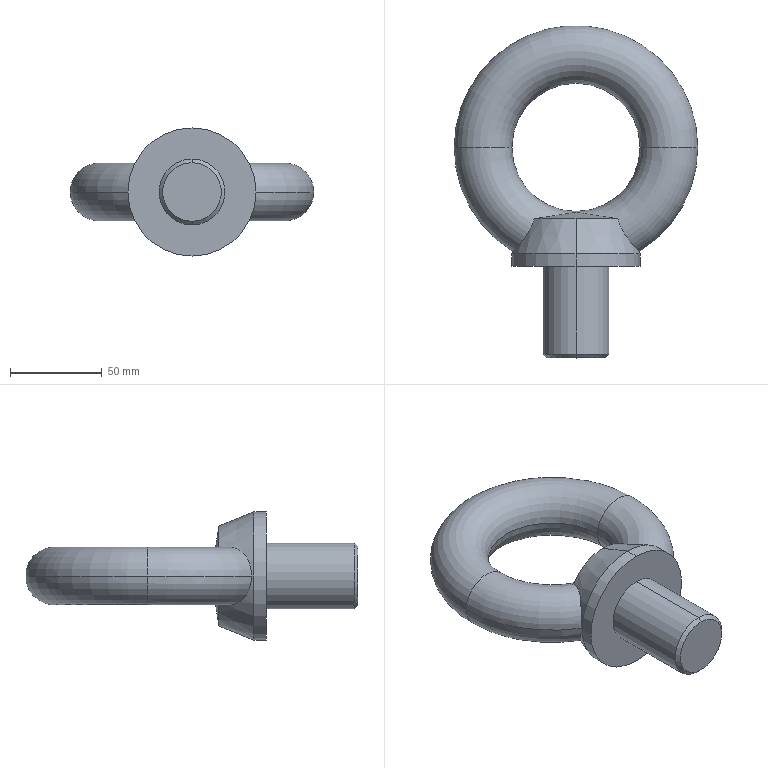Part | Creo | 1 solid | 16 faces | box 133 x 181.5 x 70 mm | volume 345866 mm3 | cone 6 | torus 4 | cylinder 4 | plane 2 | commonest cylinder face diameters 36 x2 70 x2
STEP:
#1=CARTESIAN_POINT('',(-22.859,376.,-80.242));
#2=VERTEX_POINT('',#1);
#3=CARTESIAN_POINT('',(0.,379.333,-70.034));
#4=VERTEX_POINT('',#3);
#5=CARTESIAN_POINT('',(-22.859,376.,-80.242));
#6=CARTESIAN_POINT('',(-21.93,376.132,-80.022));
#7=CARTESIAN_POINT('',(-20.175,376.386,-79.542));
#8=CARTESIAN_POINT('',(-17.843,376.731,-78.764));
#9=CARTESIAN_POINT('',(-15.766,377.045,-77.963));
#10=CARTESIAN_POINT('',(-13.906,377.331,-77.165));
#11=CARTESIAN_POINT('',(-12.241,377.591,-76.387));
#12=CARTESIAN_POINT('',(-10.742,377.828,-75.639));
#13=CARTESIAN_POINT('',(-9.385,378.044,-74.925));
#14=CARTESIAN_POINT('',(-8.149,378.242,-74.246));
#15=CARTESIAN_POINT('',(-7.011,378.425,-73.6));
#16=CARTESIAN_POINT('',(-5.956,378.594,-72.984));
#17=CARTESIAN_POINT('',(-4.977,378.75,-72.398));
#18=CARTESIAN_POINT('',(-4.073,378.891,-71.851));
#19=CARTESIAN_POINT('',(-3.245,379.016,-71.359));
#20=CARTESIAN_POINT('',(-2.502,379.122,-70.928));
#21=CARTESIAN_POINT('',(-1.815,379.213,-70.544));
#22=CARTESIAN_POINT('',(-1.153,379.284,-70.244));
#23=CARTESIAN_POINT('',(-0.5447,379.325,-70.071));
#24=CARTESIAN_POINT('',(-0.1835,379.333,-70.034));
#25=B_SPLINE_CURVE_WITH_KNOTS('',3,(#5,#6,#7,#8,#9,#10,#11,#12,#13,#14,#15,#16,#17,#18,#19,#20,#21,#22,#23,#24,#3),.UNSPECIFIED.,.F.,.F.,(4,1,1,1,1,1,1,1,1,1,1,1,1,1,1,1,1,1,4),(0.,0.05556,0.1111,0.1667,0.2222,0.2778,0.3333,0.3889,0.4444,0.5,0.5556,0.6111,0.6667,0.7222,0.7778,0.8333,0.8889,0.9444,1.),.UNSPECIFIED.);
#26=EDGE_CURVE('',#2,#4,#25,.T.);
#27=ORIENTED_EDGE('',*,*,#26,.F.);
#28=CARTESIAN_POINT('',(0.,376.,-92.7));
#29=VERTEX_POINT('',#28);
#30=CARTESIAN_POINT('',(0.,376.,-65.5));
#31=DIRECTION('',(0.,-1.,0.));
#32=DIRECTION('',(-0.8404,0.,-0.542));
#33=AXIS2_PLACEMENT_3D('',#30,#31,#32);
#34=CIRCLE('',#33,27.2);
#35=EDGE_CURVE('',#2,#29,#34,.T.);
#36=ORIENTED_EDGE('',*,*,#35,.T.);
#37=CARTESIAN_POINT('',(22.859,376.,-80.242));
#38=VERTEX_POINT('',#37);
#39=CARTESIAN_POINT('',(0.,376.,-65.5));
#40=DIRECTION('',(0.,-1.,0.));
#41=DIRECTION('',(0.,0.,-1.));
#42=AXIS2_PLACEMENT_3D('',#39,#40,#41);
#43=CIRCLE('',#42,27.2);
#44=EDGE_CURVE('',#29,#38,#43,.T.);
#45=ORIENTED_EDGE('',*,*,#44,.T.);
#46=CARTESIAN_POINT('',(0.,379.333,-70.034));
#47=CARTESIAN_POINT('',(0.1802,379.333,-70.034));
#48=CARTESIAN_POINT('',(0.5342,379.325,-70.071));
#49=CARTESIAN_POINT('',(1.137,379.283,-70.25));
#50=CARTESIAN_POINT('',(1.772,379.216,-70.538));
#51=CARTESIAN_POINT('',(2.453,379.129,-70.899));
#52=CARTESIAN_POINT('',(3.203,379.022,-71.335));
#53=CARTESIAN_POINT('',(4.029,378.898,-71.826));
#54=CARTESIAN_POINT('',(4.932,378.757,-72.37));
#55=CARTESIAN_POINT('',(5.909,378.601,-72.956));
#56=CARTESIAN_POINT('',(6.96,378.433,-73.571));
#57=CARTESIAN_POINT('',(8.095,378.251,-74.217));
#58=CARTESIAN_POINT('',(9.329,378.053,-74.896));
#59=CARTESIAN_POINT('',(10.686,377.837,-75.611));
#60=CARTESIAN_POINT('',(12.188,377.6,-76.362));
#61=CARTESIAN_POINT('',(13.857,377.339,-77.144));
#62=CARTESIAN_POINT('',(15.725,377.051,-77.948));
#63=CARTESIAN_POINT('',(17.811,376.736,-78.754));
#64=CARTESIAN_POINT('',(20.155,376.389,-79.537));
#65=CARTESIAN_POINT('',(21.923,376.133,-80.021));
#66=CARTESIAN_POINT('',(22.859,376.,-80.242));
#67=B_SPLINE_CURVE_WITH_KNOTS('',3,(#46,#47,#48,#49,#50,#51,#52,#53,#54,#55,#56,#57,#58,#59,#60,#61,#62,#63,#64,#65,#66),.UNSPECIFIED.,.F.,.F.,(4,1,1,1,1,1,1,1,1,1,1,1,1,1,1,1,1,1,4),(0.,0.05556,0.1111,0.1667,0.2222,0.2778,0.3333,0.3889,0.4444,0.5,0.5556,0.6111,0.6667,0.7222,0.7778,0.8333,0.8889,0.9444,1.),.UNSPECIFIED.);
#68=EDGE_CURVE('',#4,#38,#67,.T.);
#69=ORIENTED_EDGE('',*,*,#68,.F.);
#70=EDGE_LOOP('',(#27,#36,#45,#69));
#71=FACE_OUTER_BOUND('',#70,.F.);
#72=CARTESIAN_POINT('',(0.,377.667,-65.5));
#73=DIRECTION('',(0.,-1.,0.));
#74=DIRECTION('',(0.,0.,-1.));
#75=AXIS2_PLACEMENT_3D('',#72,#73,#74);
#76=CONICAL_SURFACE('',#75,15.867,81.634);
#77=ADVANCED_FACE('',(#71),#76,.T.);
#78=CARTESIAN_POINT('',(34.464,358.128,-65.5));
#79=VERTEX_POINT('',#78);
#80=CARTESIAN_POINT('',(22.859,376.,-80.242));
#81=CARTESIAN_POINT('',(23.041,375.255,-80.518));
#82=CARTESIAN_POINT('',(23.475,373.76,-80.963));
#83=CARTESIAN_POINT('',(24.371,371.476,-81.291));
#84=CARTESIAN_POINT('',(25.482,369.249,-81.233));
#85=CARTESIAN_POINT('',(26.763,367.124,-80.777));
#86=CARTESIAN_POINT('',(28.132,365.163,-79.93));
#87=CARTESIAN_POINT('',(29.531,363.381,-78.699));
#88=CARTESIAN_POINT('',(30.873,361.82,-77.114));
#89=CARTESIAN_POINT('',(32.081,360.511,-75.22));
#90=CARTESIAN_POINT('',(33.099,359.464,-73.055));
#91=CARTESIAN_POINT('',(33.871,358.7,-70.672));
#92=CARTESIAN_POINT('',(34.354,358.233,-68.128));
#93=CARTESIAN_POINT('',(34.464,358.128,-66.381));
#94=CARTESIAN_POINT('',(34.464,358.128,-65.5));
#95=B_SPLINE_CURVE_WITH_KNOTS('',3,(#80,#81,#82,#83,#84,#85,#86,#87,#88,#89,#90,#91,#92,#93,#94),.UNSPECIFIED.,.F.,.F.,(4,1,1,1,1,1,1,1,1,1,1,1,4),(0.,0.08333,0.1667,0.25,0.3333,0.4167,0.5,0.5833,0.6667,0.75,0.8333,0.9167,1.),.UNSPECIFIED.);
#96=EDGE_CURVE('',#38,#79,#95,.T.);
#97=ORIENTED_EDGE('',*,*,#96,.T.);
#98=CARTESIAN_POINT('',(66.5,415.,-65.5));
#99=VERTEX_POINT('',#98);
#100=CARTESIAN_POINT('',(0.,415.,-65.5));
#101=DIRECTION('',(0.,0.,1.));
#102=DIRECTION('',(0.5183,-0.8552,0.));
#103=AXIS2_PLACEMENT_3D('',#100,#101,#102);
#104=CIRCLE('',#103,66.5);
#105=EDGE_CURVE('',#79,#99,#104,.T.);
#106=ORIENTED_EDGE('',*,*,#105,.T.);
#107=CARTESIAN_POINT('',(35.,415.,-65.5));
#108=VERTEX_POINT('',#107);
#109=CARTESIAN_POINT('',(50.75,415.,-65.5));
#110=DIRECTION('',(0.,-1.,0.));
#111=DIRECTION('',(-1.,0.,0.));
#112=AXIS2_PLACEMENT_3D('',#109,#110,#111);
#113=CIRCLE('',#112,15.75);
#114=EDGE_CURVE('',#108,#99,#113,.T.);
#115=ORIENTED_EDGE('',*,*,#114,.F.);
#116=CARTESIAN_POINT('',(-35.,415.,-65.5));
#117=VERTEX_POINT('',#116);
#118=CARTESIAN_POINT('',(0.,415.,-65.5));
#119=DIRECTION('',(0.,0.,1.));
#120=DIRECTION('',(-1.,0.,0.));
#121=AXIS2_PLACEMENT_3D('',#118,#119,#120);
#122=CIRCLE('',#121,35.);
#123=EDGE_CURVE('',#117,#108,#122,.T.);
#124=ORIENTED_EDGE('',*,*,#123,.F.);
#125=CARTESIAN_POINT('',(-66.5,415.,-65.5));
#126=VERTEX_POINT('',#125);
#127=CARTESIAN_POINT('',(-50.75,415.,-65.5));
#128=DIRECTION('',(0.,1.,0.));
#129=DIRECTION('',(1.,0.,0.));
#130=AXIS2_PLACEMENT_3D('',#127,#128,#129);
#131=CIRCLE('',#130,15.75);
#132=EDGE_CURVE('',#117,#126,#131,.T.);
#133=ORIENTED_EDGE('',*,*,#132,.T.);
#134=CARTESIAN_POINT('',(-34.464,358.128,-65.5));
#135=VERTEX_POINT('',#134);
#136=CARTESIAN_POINT('',(0.,415.,-65.5));
#137=DIRECTION('',(0.,0.,1.));
#138=DIRECTION('',(-1.,0.,0.));
#139=AXIS2_PLACEMENT_3D('',#136,#137,#138);
#140=CIRCLE('',#139,66.5);
#141=EDGE_CURVE('',#126,#135,#140,.T.);
#142=ORIENTED_EDGE('',*,*,#141,.T.);
#143=CARTESIAN_POINT('',(-34.464,358.128,-65.5));
#144=CARTESIAN_POINT('',(-34.464,358.128,-66.375));
#145=CARTESIAN_POINT('',(-34.356,358.232,-68.112));
#146=CARTESIAN_POINT('',(-33.877,358.694,-70.647));
#147=CARTESIAN_POINT('',(-33.11,359.453,-73.027));
#148=CARTESIAN_POINT('',(-32.096,360.495,-75.192));
#149=CARTESIAN_POINT('',(-30.893,361.798,-77.086));
#150=CARTESIAN_POINT('',(-29.558,363.349,-78.672));
#151=CARTESIAN_POINT('',(-28.158,365.129,-79.912));
#152=CARTESIAN_POINT('',(-26.777,367.1,-80.771));
#153=CARTESIAN_POINT('',(-25.488,369.238,-81.232));
#154=CARTESIAN_POINT('',(-24.374,371.47,-81.291));
#155=CARTESIAN_POINT('',(-23.476,373.757,-80.964));
#156=CARTESIAN_POINT('',(-23.041,375.253,-80.519));
#157=CARTESIAN_POINT('',(-22.859,376.,-80.242));
#158=B_SPLINE_CURVE_WITH_KNOTS('',3,(#143,#144,#145,#146,#147,#148,#149,#150,#151,#152,#153,#154,#155,#156,#157),.UNSPECIFIED.,.F.,.F.,(4,1,1,1,1,1,1,1,1,1,1,1,4),(0.,0.08333,0.1667,0.25,0.3333,0.4167,0.5,0.5833,0.6667,0.75,0.8333,0.9167,1.),.UNSPECIFIED.);
#159=EDGE_CURVE('',#135,#2,#158,.T.);
#160=ORIENTED_EDGE('',*,*,#159,.T.);
#161=ORIENTED_EDGE('',*,*,#26,.T.);
#162=ORIENTED_EDGE('',*,*,#68,.T.);
#163=EDGE_LOOP('',(#97,#106,#115,#124,#133,#142,#160,#161,#162));
#164=FACE_OUTER_BOUND('',#163,.F.);
#165=CARTESIAN_POINT('',(0.,415.,-65.5));
#166=DIRECTION('',(0.,0.,1.));
#167=DIRECTION('',(1.,0.,0.));
#168=AXIS2_PLACEMENT_3D('',#165,#166,#167);
#169=TOROIDAL_SURFACE('',#168,50.75,15.75);
#170=ADVANCED_FACE('',(#164),#169,.T.);
#171=ORIENTED_EDGE('',*,*,#96,.F.);
#172=ORIENTED_EDGE('',*,*,#44,.F.);
#173=CARTESIAN_POINT('',(0.,356.81,-100.5));
#174=VERTEX_POINT('',#173);
#175=CARTESIAN_POINT('',(0.,376.,-92.7));
#176=DIRECTION('',(0.,-0.9264,-0.3765));
#177=VECTOR('',#176,20.715);
#178=LINE('',#175,#177);
#179=EDGE_CURVE('',#29,#174,#178,.T.);
#180=ORIENTED_EDGE('',*,*,#179,.T.);
#181=CARTESIAN_POINT('',(0.,356.81,-30.5));
#182=VERTEX_POINT('',#181);
#183=CARTESIAN_POINT('',(0.,356.81,-65.5));
#184=DIRECTION('',(0.,1.,0.));
#185=DIRECTION('',(0.,0.,1.));
#186=AXIS2_PLACEMENT_3D('',#183,#184,#185);
#187=CIRCLE('',#186,35.);
#188=EDGE_CURVE('',#182,#174,#187,.T.);
#189=ORIENTED_EDGE('',*,*,#188,.F.);
#190=CARTESIAN_POINT('',(0.,376.,-38.3));
#191=VERTEX_POINT('',#190);
#192=CARTESIAN_POINT('',(0.,376.,-38.3));
#193=DIRECTION('',(0.,-0.9264,0.3765));
#194=VECTOR('',#193,20.715);
#195=LINE('',#192,#194);
#196=EDGE_CURVE('',#191,#182,#195,.T.);
#197=ORIENTED_EDGE('',*,*,#196,.F.);
#198=CARTESIAN_POINT('',(22.859,376.,-50.758));
#199=VERTEX_POINT('',#198);
#200=CARTESIAN_POINT('',(0.,376.,-65.5));
#201=DIRECTION('',(0.,-1.,0.));
#202=DIRECTION('',(0.8404,0.,0.542));
#203=AXIS2_PLACEMENT_3D('',#200,#201,#202);
#204=CIRCLE('',#203,27.2);
#205=EDGE_CURVE('',#199,#191,#204,.T.);
#206=ORIENTED_EDGE('',*,*,#205,.F.);
#207=CARTESIAN_POINT('',(34.464,358.128,-65.5));
#208=CARTESIAN_POINT('',(34.464,358.128,-64.625));
#209=CARTESIAN_POINT('',(34.356,358.232,-62.888));
#210=CARTESIAN_POINT('',(33.877,358.694,-60.353));
#211=CARTESIAN_POINT('',(33.11,359.453,-57.973));
#212=CARTESIAN_POINT('',(32.096,360.495,-55.808));
#213=CARTESIAN_POINT('',(30.893,361.798,-53.914));
#214=CARTESIAN_POINT('',(29.558,363.349,-52.328));
#215=CARTESIAN_POINT('',(28.158,365.129,-51.088));
#216=CARTESIAN_POINT('',(26.777,367.1,-50.229));
#217=CARTESIAN_POINT('',(25.488,369.238,-49.768));
#218=CARTESIAN_POINT('',(24.374,371.47,-49.709));
#219=CARTESIAN_POINT('',(23.476,373.757,-50.036));
#220=CARTESIAN_POINT('',(23.041,375.253,-50.481));
#221=CARTESIAN_POINT('',(22.859,376.,-50.758));
#222=B_SPLINE_CURVE_WITH_KNOTS('',3,(#207,#208,#209,#210,#211,#212,#213,#214,#215,#216,#217,#218,#219,#220,#221),.UNSPECIFIED.,.F.,.F.,(4,1,1,1,1,1,1,1,1,1,1,1,4),(0.,0.08333,0.1667,0.25,0.3333,0.4167,0.5,0.5833,0.6667,0.75,0.8333,0.9167,1.),.UNSPECIFIED.);
#223=EDGE_CURVE('',#79,#199,#222,.T.);
#224=ORIENTED_EDGE('',*,*,#223,.F.);
#225=EDGE_LOOP('',(#171,#172,#180,#189,#197,#206,#224));
#226=FACE_OUTER_BOUND('',#225,.F.);
#227=CARTESIAN_POINT('',(0.,366.405,-65.5));
#228=DIRECTION('',(0.,-1.,0.));
#229=DIRECTION('',(0.,0.,-1.));
#230=AXIS2_PLACEMENT_3D('',#227,#228,#229);
#231=CONICAL_SURFACE('',#230,31.1,22.12);
#232=ADVANCED_FACE('',(#226),#231,.T.);
#233=CARTESIAN_POINT('',(-22.859,376.,-50.758));
#234=VERTEX_POINT('',#233);
#235=CARTESIAN_POINT('',(0.,376.,-65.5));
#236=DIRECTION('',(0.,-1.,0.));
#237=DIRECTION('',(0.,0.,1.));
#238=AXIS2_PLACEMENT_3D('',#235,#236,#237);
#239=CIRCLE('',#238,27.2);
#240=EDGE_CURVE('',#191,#234,#239,.T.);
#241=ORIENTED_EDGE('',*,*,#240,.F.);
#242=ORIENTED_EDGE('',*,*,#196,.T.);
#243=CARTESIAN_POINT('',(0.,356.81,-65.5));
#244=DIRECTION('',(0.,1.,0.));
#245=DIRECTION('',(0.,0.,-1.));
#246=AXIS2_PLACEMENT_3D('',#243,#244,#245);
#247=CIRCLE('',#246,35.);
#248=EDGE_CURVE('',#174,#182,#247,.T.);
#249=ORIENTED_EDGE('',*,*,#248,.F.);
#250=ORIENTED_EDGE('',*,*,#179,.F.);
#251=ORIENTED_EDGE('',*,*,#35,.F.);
#252=ORIENTED_EDGE('',*,*,#159,.F.);
#253=CARTESIAN_POINT('',(-22.859,376.,-50.758));
#254=CARTESIAN_POINT('',(-23.041,375.255,-50.482));
#255=CARTESIAN_POINT('',(-23.475,373.76,-50.037));
#256=CARTESIAN_POINT('',(-24.371,371.476,-49.709));
#257=CARTESIAN_POINT('',(-25.482,369.249,-49.767));
#258=CARTESIAN_POINT('',(-26.763,367.124,-50.223));
#259=CARTESIAN_POINT('',(-28.132,365.163,-51.07));
#260=CARTESIAN_POINT('',(-29.531,363.381,-52.301));
#261=CARTESIAN_POINT('',(-30.873,361.82,-53.886));
#262=CARTESIAN_POINT('',(-32.081,360.511,-55.78));
#263=CARTESIAN_POINT('',(-33.099,359.464,-57.945));
#264=CARTESIAN_POINT('',(-33.871,358.7,-60.328));
#265=CARTESIAN_POINT('',(-34.354,358.233,-62.872));
#266=CARTESIAN_POINT('',(-34.464,358.128,-64.619));
#267=CARTESIAN_POINT('',(-34.464,358.128,-65.5));
#268=B_SPLINE_CURVE_WITH_KNOTS('',3,(#253,#254,#255,#256,#257,#258,#259,#260,#261,#262,#263,#264,#265,#266,#267),.UNSPECIFIED.,.F.,.F.,(4,1,1,1,1,1,1,1,1,1,1,1,4),(0.,0.08333,0.1667,0.25,0.3333,0.4167,0.5,0.5833,0.6667,0.75,0.8333,0.9167,1.),.UNSPECIFIED.);
#269=EDGE_CURVE('',#234,#135,#268,.T.);
#270=ORIENTED_EDGE('',*,*,#269,.F.);
#271=EDGE_LOOP('',(#241,#242,#249,#250,#251,#252,#270));
#272=FACE_OUTER_BOUND('',#271,.F.);
#273=CARTESIAN_POINT('',(0.,366.405,-65.5));
#274=DIRECTION('',(0.,-1.,0.));
#275=DIRECTION('',(0.,0.,-1.));
#276=AXIS2_PLACEMENT_3D('',#273,#274,#275);
#277=CONICAL_SURFACE('',#276,31.1,22.12);
#278=ADVANCED_FACE('',(#272),#277,.T.);
#279=CARTESIAN_POINT('',(0.,379.333,-60.966));
#280=VERTEX_POINT('',#279);
#281=CARTESIAN_POINT('',(22.859,376.,-50.758));
#282=CARTESIAN_POINT('',(21.93,376.132,-50.978));
#283=CARTESIAN_POINT('',(20.175,376.386,-51.458));
#284=CARTESIAN_POINT('',(17.843,376.731,-52.236));
#285=CARTESIAN_POINT('',(15.766,377.045,-53.037));
#286=CARTESIAN_POINT('',(13.906,377.331,-53.835));
#287=CARTESIAN_POINT('',(12.241,377.591,-54.613));
#288=CARTESIAN_POINT('',(10.742,377.828,-55.361));
#289=CARTESIAN_POINT('',(9.385,378.044,-56.075));
#290=CARTESIAN_POINT('',(8.149,378.242,-56.754));
#291=CARTESIAN_POINT('',(7.011,378.425,-57.4));
#292=CARTESIAN_POINT('',(5.956,378.594,-58.016));
#293=CARTESIAN_POINT('',(4.977,378.75,-58.602));
#294=CARTESIAN_POINT('',(4.073,378.891,-59.149));
#295=CARTESIAN_POINT('',(3.245,379.016,-59.641));
#296=CARTESIAN_POINT('',(2.502,379.122,-60.072));
#297=CARTESIAN_POINT('',(1.815,379.213,-60.456));
#298=CARTESIAN_POINT('',(1.153,379.284,-60.756));
#299=CARTESIAN_POINT('',(0.5447,379.325,-60.929));
#300=CARTESIAN_POINT('',(0.1835,379.333,-60.966));
#301=B_SPLINE_CURVE_WITH_KNOTS('',3,(#281,#282,#283,#284,#285,#286,#287,#288,#289,#290,#291,#292,#293,#294,#295,#296,#297,#298,#299,#300,#279),.UNSPECIFIED.,.F.,.F.,(4,1,1,1,1,1,1,1,1,1,1,1,1,1,1,1,1,1,4),(0.,0.05556,0.1111,0.1667,0.2222,0.2778,0.3333,0.3889,0.4444,0.5,0.5556,0.6111,0.6667,0.7222,0.7778,0.8333,0.8889,0.9444,1.),.UNSPECIFIED.);
#302=EDGE_CURVE('',#199,#280,#301,.T.);
#303=ORIENTED_EDGE('',*,*,#302,.F.);
#304=ORIENTED_EDGE('',*,*,#205,.T.);
#305=ORIENTED_EDGE('',*,*,#240,.T.);
#306=CARTESIAN_POINT('',(0.,379.333,-60.966));
#307=CARTESIAN_POINT('',(-0.1802,379.333,-60.966));
#308=CARTESIAN_POINT('',(-0.5342,379.325,-60.929));
#309=CARTESIAN_POINT('',(-1.137,379.283,-60.75));
#310=CARTESIAN_POINT('',(-1.772,379.216,-60.462));
#311=CARTESIAN_POINT('',(-2.453,379.129,-60.101));
#312=CARTESIAN_POINT('',(-3.203,379.022,-59.665));
#313=CARTESIAN_POINT('',(-4.029,378.898,-59.174));
#314=CARTESIAN_POINT('',(-4.932,378.757,-58.63));
#315=CARTESIAN_POINT('',(-5.909,378.601,-58.044));
#316=CARTESIAN_POINT('',(-6.96,378.433,-57.429));
#317=CARTESIAN_POINT('',(-8.095,378.251,-56.783));
#318=CARTESIAN_POINT('',(-9.329,378.053,-56.104));
#319=CARTESIAN_POINT('',(-10.686,377.837,-55.389));
#320=CARTESIAN_POINT('',(-12.188,377.6,-54.638));
#321=CARTESIAN_POINT('',(-13.857,377.339,-53.856));
#322=CARTESIAN_POINT('',(-15.725,377.051,-53.052));
#323=CARTESIAN_POINT('',(-17.811,376.736,-52.246));
#324=CARTESIAN_POINT('',(-20.155,376.389,-51.463));
#325=CARTESIAN_POINT('',(-21.923,376.133,-50.979));
#326=CARTESIAN_POINT('',(-22.859,376.,-50.758));
#327=B_SPLINE_CURVE_WITH_KNOTS('',3,(#306,#307,#308,#309,#310,#311,#312,#313,#314,#315,#316,#317,#318,#319,#320,#321,#322,#323,#324,#325,#326),.UNSPECIFIED.,.F.,.F.,(4,1,1,1,1,1,1,1,1,1,1,1,1,1,1,1,1,1,4),(0.,0.05556,0.1111,0.1667,0.2222,0.2778,0.3333,0.3889,0.4444,0.5,0.5556,0.6111,0.6667,0.7222,0.7778,0.8333,0.8889,0.9444,1.),.UNSPECIFIED.);
#328=EDGE_CURVE('',#280,#234,#327,.T.);
#329=ORIENTED_EDGE('',*,*,#328,.F.);
#330=EDGE_LOOP('',(#303,#304,#305,#329));
#331=FACE_OUTER_BOUND('',#330,.F.);
#332=CARTESIAN_POINT('',(0.,377.667,-65.5));
#333=DIRECTION('',(0.,-1.,0.));
#334=DIRECTION('',(0.,0.,-1.));
#335=AXIS2_PLACEMENT_3D('',#332,#333,#334);
#336=CONICAL_SURFACE('',#335,15.867,81.634);
#337=ADVANCED_FACE('',(#331),#336,.T.);
#338=ORIENTED_EDGE('',*,*,#223,.T.);
#339=ORIENTED_EDGE('',*,*,#302,.T.);
#340=ORIENTED_EDGE('',*,*,#328,.T.);
#341=ORIENTED_EDGE('',*,*,#269,.T.);
#342=ORIENTED_EDGE('',*,*,#141,.F.);
#343=CARTESIAN_POINT('',(-50.75,415.,-65.5));
#344=DIRECTION('',(0.,1.,0.));
#345=DIRECTION('',(-1.,0.,0.));
#346=AXIS2_PLACEMENT_3D('',#343,#344,#345);
#347=CIRCLE('',#346,15.75);
#348=EDGE_CURVE('',#126,#117,#347,.T.);
#349=ORIENTED_EDGE('',*,*,#348,.T.);
#350=ORIENTED_EDGE('',*,*,#123,.T.);
#351=CARTESIAN_POINT('',(50.75,415.,-65.5));
#352=DIRECTION('',(0.,-1.,0.));
#353=DIRECTION('',(1.,0.,0.));
#354=AXIS2_PLACEMENT_3D('',#351,#352,#353);
#355=CIRCLE('',#354,15.75);
#356=EDGE_CURVE('',#99,#108,#355,.T.);
#357=ORIENTED_EDGE('',*,*,#356,.F.);
#358=ORIENTED_EDGE('',*,*,#105,.F.);
#359=EDGE_LOOP('',(#338,#339,#340,#341,#342,#349,#350,#357,#358));
#360=FACE_OUTER_BOUND('',#359,.F.);
#361=CARTESIAN_POINT('',(0.,415.,-65.5));
#362=DIRECTION('',(0.,0.,1.));
#363=DIRECTION('',(1.,0.,0.));
#364=AXIS2_PLACEMENT_3D('',#361,#362,#363);
#365=TOROIDAL_SURFACE('',#364,50.75,15.75);
#366=ADVANCED_FACE('',(#360),#365,.T.);
#367=CARTESIAN_POINT('',(0.,415.,-65.5));
#368=DIRECTION('',(0.,0.,1.));
#369=DIRECTION('',(1.,0.,0.));
#370=AXIS2_PLACEMENT_3D('',#367,#368,#369);
#371=CIRCLE('',#370,66.5);
#372=EDGE_CURVE('',#99,#126,#371,.T.);
#373=ORIENTED_EDGE('',*,*,#372,.F.);
#374=ORIENTED_EDGE('',*,*,#356,.T.);
#375=CARTESIAN_POINT('',(0.,415.,-65.5));
#376=DIRECTION('',(0.,0.,1.));
#377=DIRECTION('',(1.,0.,0.));
#378=AXIS2_PLACEMENT_3D('',#375,#376,#377);
#379=CIRCLE('',#378,35.);
#380=EDGE_CURVE('',#108,#117,#379,.T.);
#381=ORIENTED_EDGE('',*,*,#380,.T.);
#382=ORIENTED_EDGE('',*,*,#348,.F.);
#383=EDGE_LOOP('',(#373,#374,#381,#382));
#384=FACE_OUTER_BOUND('',#383,.F.);
#385=CARTESIAN_POINT('',(0.,415.,-65.5));
#386=DIRECTION('',(0.,0.,1.));
#387=DIRECTION('',(1.,0.,0.));
#388=AXIS2_PLACEMENT_3D('',#385,#386,#387);
#389=TOROIDAL_SURFACE('',#388,50.75,15.75);
#390=ADVANCED_FACE('',(#384),#389,.T.);
#391=ORIENTED_EDGE('',*,*,#380,.F.);
#392=ORIENTED_EDGE('',*,*,#114,.T.);
#393=ORIENTED_EDGE('',*,*,#372,.T.);
#394=ORIENTED_EDGE('',*,*,#132,.F.);
#395=EDGE_LOOP('',(#391,#392,#393,#394));
#396=FACE_OUTER_BOUND('',#395,.F.);
#397=CARTESIAN_POINT('',(0.,415.,-65.5));
#398=DIRECTION('',(0.,0.,1.));
#399=DIRECTION('',(1.,0.,0.));
#400=AXIS2_PLACEMENT_3D('',#397,#398,#399);
#401=TOROIDAL_SURFACE('',#400,50.75,15.75);
#402=ADVANCED_FACE('',(#396),#401,.T.);
#403=ORIENTED_EDGE('',*,*,#248,.T.);
#404=CARTESIAN_POINT('',(0.,350.,-30.5));
#405=VERTEX_POINT('',#404);
#406=CARTESIAN_POINT('',(0.,350.,-30.5));
#407=DIRECTION('',(0.,1.,0.));
#408=VECTOR('',#407,6.81);
#409=LINE('',#406,#408);
#410=EDGE_CURVE('',#405,#182,#409,.T.);
#411=ORIENTED_EDGE('',*,*,#410,.F.);
#412=CARTESIAN_POINT('',(0.,350.,-100.5));
#413=VERTEX_POINT('',#412);
#414=CARTESIAN_POINT('',(0.,350.,-65.5));
#415=DIRECTION('',(0.,-1.,0.));
#416=DIRECTION('',(0.,0.,1.));
#417=AXIS2_PLACEMENT_3D('',#414,#415,#416);
#418=CIRCLE('',#417,35.);
#419=EDGE_CURVE('',#405,#413,#418,.T.);
#420=ORIENTED_EDGE('',*,*,#419,.T.);
#421=CARTESIAN_POINT('',(0.,350.,-100.5));
#422=DIRECTION('',(0.,1.,0.));
#423=VECTOR('',#422,6.81);
#424=LINE('',#421,#423);
#425=EDGE_CURVE('',#413,#174,#424,.T.);
#426=ORIENTED_EDGE('',*,*,#425,.T.);
#427=EDGE_LOOP('',(#403,#411,#420,#426));
#428=FACE_OUTER_BOUND('',#427,.F.);
#429=CARTESIAN_POINT('',(0.,350.,-65.5));
#430=DIRECTION('',(0.,1.,0.));
#431=DIRECTION('',(0.,0.,1.));
#432=AXIS2_PLACEMENT_3D('',#429,#430,#431);
#433=CYLINDRICAL_SURFACE('',#432,35.);
#434=ADVANCED_FACE('',(#428),#433,.T.);
#435=ORIENTED_EDGE('',*,*,#188,.T.);
#436=ORIENTED_EDGE('',*,*,#425,.F.);
#437=CARTESIAN_POINT('',(0.,350.,-65.5));
#438=DIRECTION('',(0.,-1.,0.));
#439=DIRECTION('',(0.,0.,-1.));
#440=AXIS2_PLACEMENT_3D('',#437,#438,#439);
#441=CIRCLE('',#440,35.);
#442=EDGE_CURVE('',#413,#405,#441,.T.);
#443=ORIENTED_EDGE('',*,*,#442,.T.);
#444=ORIENTED_EDGE('',*,*,#410,.T.);
#445=EDGE_LOOP('',(#435,#436,#443,#444));
#446=FACE_OUTER_BOUND('',#445,.F.);
#447=CARTESIAN_POINT('',(0.,350.,-65.5));
#448=DIRECTION('',(0.,1.,0.));
#449=DIRECTION('',(0.,0.,1.));
#450=AXIS2_PLACEMENT_3D('',#447,#448,#449);
#451=CYLINDRICAL_SURFACE('',#450,35.);
#452=ADVANCED_FACE('',(#446),#451,.T.);
#453=ORIENTED_EDGE('',*,*,#419,.F.);
#454=ORIENTED_EDGE('',*,*,#442,.F.);
#455=EDGE_LOOP('',(#453,#454));
#456=FACE_OUTER_BOUND('',#455,.F.);
#457=CARTESIAN_POINT('',(0.,350.,-83.5));
#458=VERTEX_POINT('',#457);
#459=CARTESIAN_POINT('',(0.,350.,-47.5));
#460=VERTEX_POINT('',#459);
#461=CARTESIAN_POINT('',(0.,350.,-65.5));
#462=DIRECTION('',(0.,1.,0.));
#463=DIRECTION('',(0.,0.,-1.));
#464=AXIS2_PLACEMENT_3D('',#461,#462,#463);
#465=CIRCLE('',#464,18.);
#466=EDGE_CURVE('',#458,#460,#465,.T.);
#467=ORIENTED_EDGE('',*,*,#466,.F.);
#468=CARTESIAN_POINT('',(0.,350.,-65.5));
#469=DIRECTION('',(0.,1.,0.));
#470=DIRECTION('',(0.,0.,1.));
#471=AXIS2_PLACEMENT_3D('',#468,#469,#470);
#472=CIRCLE('',#471,18.);
#473=EDGE_CURVE('',#460,#458,#472,.T.);
#474=ORIENTED_EDGE('',*,*,#473,.F.);
#475=EDGE_LOOP('',(#467,#474));
#476=FACE_BOUND('',#475,.F.);
#477=CARTESIAN_POINT('',(0.,350.,-65.5));
#478=DIRECTION('',(0.,-1.,0.));
#479=DIRECTION('',(0.,0.,-1.));
#480=AXIS2_PLACEMENT_3D('',#477,#478,#479);
#481=PLANE('',#480);
#482=ADVANCED_FACE('',(#456,#476),#481,.T.);
#483=ORIENTED_EDGE('',*,*,#466,.T.);
#484=CARTESIAN_POINT('',(0.,302.,-47.5));
#485=VERTEX_POINT('',#484);
#486=CARTESIAN_POINT('',(0.,302.,-47.5));
#487=DIRECTION('',(0.,1.,0.));
#488=VECTOR('',#487,48.);
#489=LINE('',#486,#488);
#490=EDGE_CURVE('',#485,#460,#489,.T.);
#491=ORIENTED_EDGE('',*,*,#490,.F.);
#492=CARTESIAN_POINT('',(0.,302.,-83.5));
#493=VERTEX_POINT('',#492);
#494=CARTESIAN_POINT('',(0.,302.,-65.5));
#495=DIRECTION('',(0.,-1.,0.));
#496=DIRECTION('',(0.,0.,1.));
#497=AXIS2_PLACEMENT_3D('',#494,#495,#496);
#498=CIRCLE('',#497,18.);
#499=EDGE_CURVE('',#485,#493,#498,.T.);
#500=ORIENTED_EDGE('',*,*,#499,.T.);
#501=CARTESIAN_POINT('',(0.,302.,-83.5));
#502=DIRECTION('',(0.,1.,0.));
#503=VECTOR('',#502,48.);
#504=LINE('',#501,#503);
#505=EDGE_CURVE('',#493,#458,#504,.T.);
#506=ORIENTED_EDGE('',*,*,#505,.T.);
#507=EDGE_LOOP('',(#483,#491,#500,#506));
#508=FACE_OUTER_BOUND('',#507,.F.);
#509=CARTESIAN_POINT('',(0.,302.,-65.5));
#510=DIRECTION('',(0.,1.,0.));
#511=DIRECTION('',(0.,0.,1.));
#512=AXIS2_PLACEMENT_3D('',#509,#510,#511);
#513=CYLINDRICAL_SURFACE('',#512,18.);
#514=ADVANCED_FACE('',(#508),#513,.T.);
#515=ORIENTED_EDGE('',*,*,#473,.T.);
#516=ORIENTED_EDGE('',*,*,#505,.F.);
#517=CARTESIAN_POINT('',(0.,302.,-65.5));
#518=DIRECTION('',(0.,-1.,0.));
#519=DIRECTION('',(0.,0.,-1.));
#520=AXIS2_PLACEMENT_3D('',#517,#518,#519);
#521=CIRCLE('',#520,18.);
#522=EDGE_CURVE('',#493,#485,#521,.T.);
#523=ORIENTED_EDGE('',*,*,#522,.T.);
#524=ORIENTED_EDGE('',*,*,#490,.T.);
#525=EDGE_LOOP('',(#515,#516,#523,#524));
#526=FACE_OUTER_BOUND('',#525,.F.);
#527=CARTESIAN_POINT('',(0.,302.,-65.5));
#528=DIRECTION('',(0.,1.,0.));
#529=DIRECTION('',(0.,0.,1.));
#530=AXIS2_PLACEMENT_3D('',#527,#528,#529);
#531=CYLINDRICAL_SURFACE('',#530,18.);
#532=ADVANCED_FACE('',(#526),#531,.T.);
#533=CARTESIAN_POINT('',(0.,300.,-81.5));
#534=VERTEX_POINT('',#533);
#535=CARTESIAN_POINT('',(0.,300.,-49.5));
#536=VERTEX_POINT('',#535);
#537=CARTESIAN_POINT('',(0.,300.,-65.5));
#538=DIRECTION('',(0.,-1.,0.));
#539=DIRECTION('',(0.,0.,-1.));
#540=AXIS2_PLACEMENT_3D('',#537,#538,#539);
#541=CIRCLE('',#540,16.);
#542=EDGE_CURVE('',#534,#536,#541,.T.);
#543=ORIENTED_EDGE('',*,*,#542,.T.);
#544=CARTESIAN_POINT('',(0.,300.,-49.5));
#545=DIRECTION('',(0.,0.7071,0.7071));
#546=VECTOR('',#545,2.828);
#547=LINE('',#544,#546);
#548=EDGE_CURVE('',#536,#485,#547,.T.);
#549=ORIENTED_EDGE('',*,*,#548,.T.);
#550=ORIENTED_EDGE('',*,*,#522,.F.);
#551=CARTESIAN_POINT('',(0.,300.,-81.5));
#552=DIRECTION('',(0.,0.7071,-0.7071));
#553=VECTOR('',#552,2.828);
#554=LINE('',#551,#553);
#555=EDGE_CURVE('',#534,#493,#554,.T.);
#556=ORIENTED_EDGE('',*,*,#555,.F.);
#557=EDGE_LOOP('',(#543,#549,#550,#556));
#558=FACE_OUTER_BOUND('',#557,.F.);
#559=CARTESIAN_POINT('',(0.,301.,-65.5));
#560=DIRECTION('',(0.,1.,0.));
#561=DIRECTION('',(0.,0.,1.));
#562=AXIS2_PLACEMENT_3D('',#559,#560,#561);
#563=CONICAL_SURFACE('',#562,17.,45.);
#564=ADVANCED_FACE('',(#558),#563,.T.);
#565=CARTESIAN_POINT('',(0.,300.,-65.5));
#566=DIRECTION('',(0.,-1.,0.));
#567=DIRECTION('',(0.,0.,1.));
#568=AXIS2_PLACEMENT_3D('',#565,#566,#567);
#569=CIRCLE('',#568,16.);
#570=EDGE_CURVE('',#536,#534,#569,.T.);
#571=ORIENTED_EDGE('',*,*,#570,.F.);
#572=ORIENTED_EDGE('',*,*,#542,.F.);
#573=EDGE_LOOP('',(#571,#572));
#574=FACE_OUTER_BOUND('',#573,.F.);
#575=CARTESIAN_POINT('',(0.,300.,-65.5));
#576=DIRECTION('',(0.,-1.,0.));
#577=DIRECTION('',(0.,0.,-1.));
#578=AXIS2_PLACEMENT_3D('',#575,#576,#577);
#579=PLANE('',#578);
#580=ADVANCED_FACE('',(#574),#579,.T.);
#581=ORIENTED_EDGE('',*,*,#570,.T.);
#582=ORIENTED_EDGE('',*,*,#555,.T.);
#583=ORIENTED_EDGE('',*,*,#499,.F.);
#584=ORIENTED_EDGE('',*,*,#548,.F.);
#585=EDGE_LOOP('',(#581,#582,#583,#584));
#586=FACE_OUTER_BOUND('',#585,.F.);
#587=CARTESIAN_POINT('',(0.,301.,-65.5));
#588=DIRECTION('',(0.,1.,0.));
#589=DIRECTION('',(0.,0.,1.));
#590=AXIS2_PLACEMENT_3D('',#587,#588,#589);
#591=CONICAL_SURFACE('',#590,17.,45.);
#592=ADVANCED_FACE('',(#586),#591,.T.);
#593=CLOSED_SHELL('',(#77,#170,#232,#278,#337,#366,#390,#402,#434,#452,#482,#514,#532,#564,#580,#592));
#594=MANIFOLD_SOLID_BREP('',#593);
#595=(LENGTH_UNIT()NAMED_UNIT(*)SI_UNIT(.MILLI.,.METRE.));
#596=UNCERTAINTY_MEASURE_WITH_UNIT(LENGTH_MEASURE(0.02356),#595,'','');
#597=(NAMED_UNIT(*)PLANE_ANGLE_UNIT()SI_UNIT($,.RADIAN.));
#598=PLANE_ANGLE_MEASURE_WITH_UNIT(PLANE_ANGLE_MEASURE(0.01745),#597);
#599=(CONVERSION_BASED_UNIT('DEGREE',#598)NAMED_UNIT(*)PLANE_ANGLE_UNIT());
#600=(NAMED_UNIT(*)SI_UNIT($,.STERADIAN.)SOLID_ANGLE_UNIT());
#601=(GEOMETRIC_REPRESENTATION_CONTEXT(3)GLOBAL_UNCERTAINTY_ASSIGNED_CONTEXT((#596))GLOBAL_UNIT_ASSIGNED_CONTEXT((#595,#599,#600))REPRESENTATION_CONTEXT('',''));
#602=ADVANCED_BREP_SHAPE_REPRESENTATION('',(#594),#601);